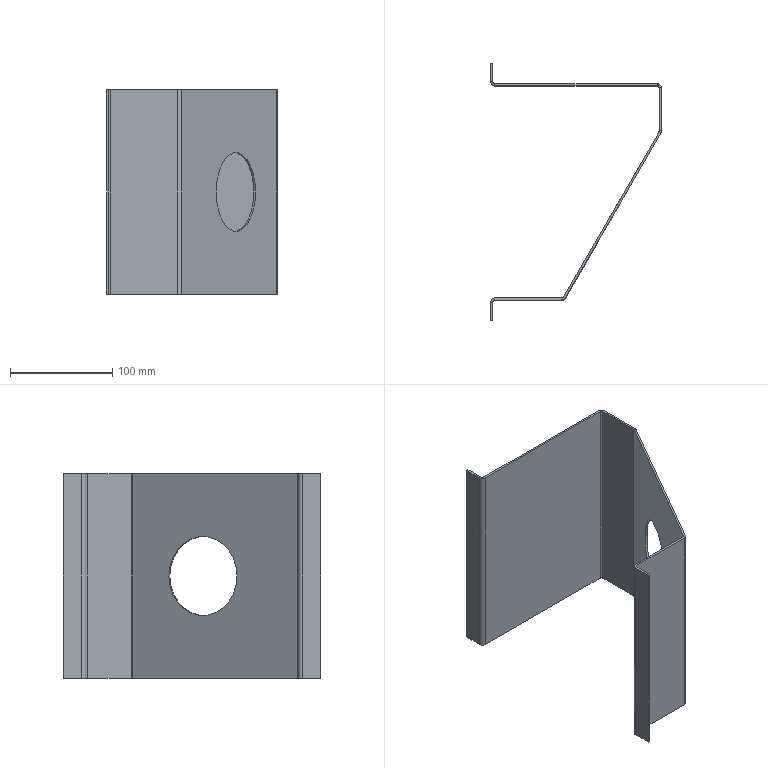Part | STEP file | SYL0380DJ1008_2_7_2_1-2_STEP | 1 solid | 48 faces | box 167 x 252 x 200 mm | volume 194104 mm3 | plane 36 | cylinder 12 | commonest cylinder face diameters 4 x5 8 x5 77 x2
STEP:
#1=CARTESIAN_POINT('',(105.214,80.993,0.));
#2=VERTEX_POINT('',#1);
#3=CARTESIAN_POINT('',(103.482,81.993,0.));
#4=VERTEX_POINT('',#3);
#5=CARTESIAN_POINT('',(103.482,81.993,0.));
#6=DIRECTION('',(-0.866,0.5,0.));
#7=VECTOR('',#6,1000.);
#8=LINE('',#5,#7);
#9=EDGE_CURVE('',#2,#4,#8,.T.);
#10=ORIENTED_EDGE('',*,*,#9,.F.);
#11=CARTESIAN_POINT('',(143.714,147.677,0.));
#12=VERTEX_POINT('',#11);
#13=CARTESIAN_POINT('',(124.464,114.335,0.));
#14=DIRECTION('',(0.866,-0.5,0.));
#15=DIRECTION('',(0.5,0.866,0.));
#16=AXIS2_PLACEMENT_3D('',#13,#14,#15);
#17=CIRCLE('',#16,38.5);
#18=EDGE_CURVE('',#2,#12,#17,.T.);
#19=ORIENTED_EDGE('',*,*,#18,.T.);
#20=CARTESIAN_POINT('',(141.982,148.677,0.));
#21=VERTEX_POINT('',#20);
#22=CARTESIAN_POINT('',(141.982,148.677,0.));
#23=DIRECTION('',(-0.866,0.5,0.));
#24=VECTOR('',#23,1000.);
#25=LINE('',#22,#24);
#26=EDGE_CURVE('',#12,#21,#25,.T.);
#27=ORIENTED_EDGE('',*,*,#26,.T.);
#28=CARTESIAN_POINT('',(122.732,115.335,0.));
#29=DIRECTION('',(0.866,-0.5,0.));
#30=DIRECTION('',(-0.5,-0.866,0.));
#31=AXIS2_PLACEMENT_3D('',#28,#29,#30);
#32=CIRCLE('',#31,38.5);
#33=EDGE_CURVE('',#4,#21,#32,.T.);
#34=ORIENTED_EDGE('',*,*,#33,.F.);
#35=EDGE_LOOP('',(#10,#19,#27,#34));
#36=FACE_OUTER_BOUND('',#35,.T.);
#37=CARTESIAN_POINT('',(122.732,115.335,0.));
#38=DIRECTION('',(0.866,-0.5,0.));
#39=DIRECTION('',(0.5,0.866,0.));
#40=AXIS2_PLACEMENT_3D('',#37,#38,#39);
#41=CYLINDRICAL_SURFACE('',#40,38.5);
#42=ADVANCED_FACE('',(#36),#41,.F.);
#43=CARTESIAN_POINT('',(161.,232.,-100.));
#44=VERTEX_POINT('',#43);
#45=CARTESIAN_POINT('',(161.,230.,-100.));
#46=VERTEX_POINT('',#45);
#47=CARTESIAN_POINT('',(161.,230.,-100.));
#48=DIRECTION('',(0.,-1.,0.));
#49=VECTOR('',#48,1000.);
#50=LINE('',#47,#49);
#51=EDGE_CURVE('',#44,#46,#50,.T.);
#52=ORIENTED_EDGE('',*,*,#51,.F.);
#53=CARTESIAN_POINT('',(165.,228.,-100.));
#54=VERTEX_POINT('',#53);
#55=CARTESIAN_POINT('',(161.,228.,-100.));
#56=DIRECTION('',(0.,0.,1.));
#57=DIRECTION('',(-1.,0.,0.));
#58=AXIS2_PLACEMENT_3D('',#55,#56,#57);
#59=CIRCLE('',#58,4.);
#60=EDGE_CURVE('',#54,#44,#59,.T.);
#61=ORIENTED_EDGE('',*,*,#60,.F.);
#62=CARTESIAN_POINT('',(163.,228.,-100.));
#63=VERTEX_POINT('',#62);
#64=CARTESIAN_POINT('',(163.,228.,-100.));
#65=DIRECTION('',(-1.,0.,0.));
#66=VECTOR('',#65,1000.);
#67=LINE('',#64,#66);
#68=EDGE_CURVE('',#54,#63,#67,.T.);
#69=ORIENTED_EDGE('',*,*,#68,.T.);
#70=CARTESIAN_POINT('',(161.,228.,-100.));
#71=DIRECTION('',(0.,0.,1.));
#72=DIRECTION('',(1.,0.,0.));
#73=AXIS2_PLACEMENT_3D('',#70,#71,#72);
#74=CIRCLE('',#73,2.);
#75=EDGE_CURVE('',#63,#46,#74,.T.);
#76=ORIENTED_EDGE('',*,*,#75,.T.);
#77=EDGE_LOOP('',(#52,#61,#69,#76));
#78=FACE_OUTER_BOUND('',#77,.T.);
#79=CARTESIAN_POINT('',(161.,228.,-100.));
#80=DIRECTION('',(0.,0.,-1.));
#81=DIRECTION('',(-1.,0.,0.));
#82=AXIS2_PLACEMENT_3D('',#79,#80,#81);
#83=PLANE('',#82);
#84=ADVANCED_FACE('',(#78),#83,.T.);
#85=ORIENTED_EDGE('',*,*,#68,.F.);
#86=CARTESIAN_POINT('',(165.,185.617,-100.));
#87=VERTEX_POINT('',#86);
#88=CARTESIAN_POINT('',(165.,184.545,-100.));
#89=DIRECTION('',(0.,-1.,0.));
#90=VECTOR('',#89,1000.);
#91=LINE('',#88,#90);
#92=EDGE_CURVE('',#54,#87,#91,.T.);
#93=ORIENTED_EDGE('',*,*,#92,.T.);
#94=CARTESIAN_POINT('',(163.,185.617,-100.));
#95=VERTEX_POINT('',#94);
#96=CARTESIAN_POINT('',(163.,185.617,-100.));
#97=DIRECTION('',(-1.,0.,0.));
#98=VECTOR('',#97,1000.);
#99=LINE('',#96,#98);
#100=EDGE_CURVE('',#87,#95,#99,.T.);
#101=ORIENTED_EDGE('',*,*,#100,.T.);
#102=CARTESIAN_POINT('',(163.,228.,-100.));
#103=DIRECTION('',(0.,-1.,0.));
#104=VECTOR('',#103,1000.);
#105=LINE('',#102,#104);
#106=EDGE_CURVE('',#63,#95,#105,.T.);
#107=ORIENTED_EDGE('',*,*,#106,.F.);
#108=EDGE_LOOP('',(#85,#93,#101,#107));
#109=FACE_OUTER_BOUND('',#108,.T.);
#110=CARTESIAN_POINT('',(163.,228.,-100.));
#111=DIRECTION('',(0.,0.,1.));
#112=DIRECTION('',(0.,-1.,0.));
#113=AXIS2_PLACEMENT_3D('',#110,#111,#112);
#114=PLANE('',#113);
#115=ADVANCED_FACE('',(#109),#114,.F.);
#116=ORIENTED_EDGE('',*,*,#100,.F.);
#117=CARTESIAN_POINT('',(164.464,183.617,-100.));
#118=VERTEX_POINT('',#117);
#119=CARTESIAN_POINT('',(161.,185.617,-100.));
#120=DIRECTION('',(0.,0.,1.));
#121=DIRECTION('',(-1.,0.,0.));
#122=AXIS2_PLACEMENT_3D('',#119,#120,#121);
#123=CIRCLE('',#122,4.);
#124=EDGE_CURVE('',#118,#87,#123,.T.);
#125=ORIENTED_EDGE('',*,*,#124,.F.);
#126=CARTESIAN_POINT('',(162.732,184.617,-100.));
#127=VERTEX_POINT('',#126);
#128=CARTESIAN_POINT('',(162.732,184.617,-100.));
#129=DIRECTION('',(-0.866,0.5,0.));
#130=VECTOR('',#129,1000.);
#131=LINE('',#128,#130);
#132=EDGE_CURVE('',#118,#127,#131,.T.);
#133=ORIENTED_EDGE('',*,*,#132,.T.);
#134=CARTESIAN_POINT('',(161.,185.617,-100.));
#135=DIRECTION('',(0.,0.,1.));
#136=DIRECTION('',(0.866,-0.5,0.));
#137=AXIS2_PLACEMENT_3D('',#134,#135,#136);
#138=CIRCLE('',#137,2.);
#139=EDGE_CURVE('',#127,#95,#138,.T.);
#140=ORIENTED_EDGE('',*,*,#139,.T.);
#141=EDGE_LOOP('',(#116,#125,#133,#140));
#142=FACE_OUTER_BOUND('',#141,.T.);
#143=CARTESIAN_POINT('',(161.,185.617,-100.));
#144=DIRECTION('',(0.,0.,-1.));
#145=DIRECTION('',(-1.,0.,0.));
#146=AXIS2_PLACEMENT_3D('',#143,#144,#145);
#147=PLANE('',#146);
#148=ADVANCED_FACE('',(#142),#147,.T.);
#149=ORIENTED_EDGE('',*,*,#132,.F.);
#150=CARTESIAN_POINT('',(71.155,22.,-100.));
#151=VERTEX_POINT('',#150);
#152=CARTESIAN_POINT('',(70.,20.,-100.));
#153=DIRECTION('',(0.5,0.866,0.));
#154=VECTOR('',#153,1000.);
#155=LINE('',#152,#154);
#156=EDGE_CURVE('',#151,#118,#155,.T.);
#157=ORIENTED_EDGE('',*,*,#156,.F.);
#158=CARTESIAN_POINT('',(69.423,23.,-100.));
#159=VERTEX_POINT('',#158);
#160=CARTESIAN_POINT('',(69.423,23.,-100.));
#161=DIRECTION('',(-0.866,0.5,0.));
#162=VECTOR('',#161,1000.);
#163=LINE('',#160,#162);
#164=EDGE_CURVE('',#151,#159,#163,.T.);
#165=ORIENTED_EDGE('',*,*,#164,.T.);
#166=CARTESIAN_POINT('',(69.423,23.,-100.));
#167=DIRECTION('',(0.5,0.866,0.));
#168=VECTOR('',#167,1000.);
#169=LINE('',#166,#168);
#170=EDGE_CURVE('',#159,#127,#169,.T.);
#171=ORIENTED_EDGE('',*,*,#170,.T.);
#172=EDGE_LOOP('',(#149,#157,#165,#171));
#173=FACE_OUTER_BOUND('',#172,.T.);
#174=CARTESIAN_POINT('',(69.423,23.,-100.));
#175=DIRECTION('',(0.,0.,-1.));
#176=DIRECTION('',(0.5,0.866,0.));
#177=AXIS2_PLACEMENT_3D('',#174,#175,#176);
#178=PLANE('',#177);
#179=ADVANCED_FACE('',(#173),#178,.T.);
#180=ORIENTED_EDGE('',*,*,#164,.F.);
#181=CARTESIAN_POINT('',(67.691,20.,-100.));
#182=VERTEX_POINT('',#181);
#183=CARTESIAN_POINT('',(67.691,24.,-100.));
#184=DIRECTION('',(0.,0.,1.));
#185=DIRECTION('',(-1.,0.,0.));
#186=AXIS2_PLACEMENT_3D('',#183,#184,#185);
#187=CIRCLE('',#186,4.);
#188=EDGE_CURVE('',#182,#151,#187,.T.);
#189=ORIENTED_EDGE('',*,*,#188,.F.);
#190=CARTESIAN_POINT('',(67.691,22.,-100.));
#191=VERTEX_POINT('',#190);
#192=CARTESIAN_POINT('',(67.691,22.,-100.));
#193=DIRECTION('',(0.,1.,0.));
#194=VECTOR('',#193,1000.);
#195=LINE('',#192,#194);
#196=EDGE_CURVE('',#182,#191,#195,.T.);
#197=ORIENTED_EDGE('',*,*,#196,.T.);
#198=CARTESIAN_POINT('',(67.691,24.,-100.));
#199=DIRECTION('',(0.,0.,1.));
#200=DIRECTION('',(0.,-1.,0.));
#201=AXIS2_PLACEMENT_3D('',#198,#199,#200);
#202=CIRCLE('',#201,2.);
#203=EDGE_CURVE('',#191,#159,#202,.T.);
#204=ORIENTED_EDGE('',*,*,#203,.T.);
#205=EDGE_LOOP('',(#180,#189,#197,#204));
#206=FACE_OUTER_BOUND('',#205,.T.);
#207=CARTESIAN_POINT('',(67.691,24.,-100.));
#208=DIRECTION('',(0.,0.,-1.));
#209=DIRECTION('',(-1.,0.,0.));
#210=AXIS2_PLACEMENT_3D('',#207,#208,#209);
#211=PLANE('',#210);
#212=ADVANCED_FACE('',(#206),#211,.T.);
#213=ORIENTED_EDGE('',*,*,#196,.F.);
#214=CARTESIAN_POINT('',(2.,20.,-100.));
#215=VERTEX_POINT('',#214);
#216=CARTESIAN_POINT('',(0.,20.,-100.));
#217=DIRECTION('',(-1.,0.,0.));
#218=VECTOR('',#217,1000.);
#219=LINE('',#216,#218);
#220=EDGE_CURVE('',#182,#215,#219,.T.);
#221=ORIENTED_EDGE('',*,*,#220,.T.);
#222=CARTESIAN_POINT('',(2.,22.,-100.));
#223=VERTEX_POINT('',#222);
#224=CARTESIAN_POINT('',(2.,22.,-100.));
#225=DIRECTION('',(0.,1.,0.));
#226=VECTOR('',#225,1000.);
#227=LINE('',#224,#226);
#228=EDGE_CURVE('',#215,#223,#227,.T.);
#229=ORIENTED_EDGE('',*,*,#228,.T.);
#230=CARTESIAN_POINT('',(67.691,22.,-100.));
#231=DIRECTION('',(-1.,0.,0.));
#232=VECTOR('',#231,1000.);
#233=LINE('',#230,#232);
#234=EDGE_CURVE('',#191,#223,#233,.T.);
#235=ORIENTED_EDGE('',*,*,#234,.F.);
#236=EDGE_LOOP('',(#213,#221,#229,#235));
#237=FACE_OUTER_BOUND('',#236,.T.);
#238=CARTESIAN_POINT('',(67.691,22.,-100.));
#239=DIRECTION('',(0.,0.,1.));
#240=DIRECTION('',(-1.,0.,0.));
#241=AXIS2_PLACEMENT_3D('',#238,#239,#240);
#242=PLANE('',#241);
#243=ADVANCED_FACE('',(#237),#242,.F.);
#244=ORIENTED_EDGE('',*,*,#228,.F.);
#245=CARTESIAN_POINT('',(0.,18.,-100.));
#246=VERTEX_POINT('',#245);
#247=CARTESIAN_POINT('',(2.,18.,-100.));
#248=DIRECTION('',(0.,0.,-1.));
#249=DIRECTION('',(1.,0.,0.));
#250=AXIS2_PLACEMENT_3D('',#247,#248,#249);
#251=CIRCLE('',#250,2.);
#252=EDGE_CURVE('',#246,#215,#251,.T.);
#253=ORIENTED_EDGE('',*,*,#252,.F.);
#254=CARTESIAN_POINT('',(-2.,18.,-100.));
#255=VERTEX_POINT('',#254);
#256=CARTESIAN_POINT('',(-2.,18.,-100.));
#257=DIRECTION('',(-1.,0.,0.));
#258=VECTOR('',#257,1000.);
#259=LINE('',#256,#258);
#260=EDGE_CURVE('',#246,#255,#259,.T.);
#261=ORIENTED_EDGE('',*,*,#260,.T.);
#262=CARTESIAN_POINT('',(2.,18.,-100.));
#263=DIRECTION('',(0.,0.,-1.));
#264=DIRECTION('',(-1.,0.,0.));
#265=AXIS2_PLACEMENT_3D('',#262,#263,#264);
#266=CIRCLE('',#265,4.);
#267=EDGE_CURVE('',#255,#223,#266,.T.);
#268=ORIENTED_EDGE('',*,*,#267,.T.);
#269=EDGE_LOOP('',(#244,#253,#261,#268));
#270=FACE_OUTER_BOUND('',#269,.T.);
#271=CARTESIAN_POINT('',(2.,18.,-100.));
#272=DIRECTION('',(0.,0.,1.));
#273=DIRECTION('',(1.,0.,0.));
#274=AXIS2_PLACEMENT_3D('',#271,#272,#273);
#275=PLANE('',#274);
#276=ADVANCED_FACE('',(#270),#275,.F.);
#277=ORIENTED_EDGE('',*,*,#260,.F.);
#278=CARTESIAN_POINT('',(0.,0.,-100.));
#279=VERTEX_POINT('',#278);
#280=CARTESIAN_POINT('',(0.,0.,-100.));
#281=DIRECTION('',(0.,-1.,0.));
#282=VECTOR('',#281,1000.);
#283=LINE('',#280,#282);
#284=EDGE_CURVE('',#246,#279,#283,.T.);
#285=ORIENTED_EDGE('',*,*,#284,.T.);
#286=CARTESIAN_POINT('',(-2.,0.,-100.));
#287=VERTEX_POINT('',#286);
#288=CARTESIAN_POINT('',(-2.,0.,-100.));
#289=DIRECTION('',(-1.,0.,0.));
#290=VECTOR('',#289,1000.);
#291=LINE('',#288,#290);
#292=EDGE_CURVE('',#279,#287,#291,.T.);
#293=ORIENTED_EDGE('',*,*,#292,.T.);
#294=CARTESIAN_POINT('',(-2.,18.,-100.));
#295=DIRECTION('',(0.,-1.,0.));
#296=VECTOR('',#295,1000.);
#297=LINE('',#294,#296);
#298=EDGE_CURVE('',#255,#287,#297,.T.);
#299=ORIENTED_EDGE('',*,*,#298,.F.);
#300=EDGE_LOOP('',(#277,#285,#293,#299));
#301=FACE_OUTER_BOUND('',#300,.T.);
#302=CARTESIAN_POINT('',(-2.,18.,-100.));
#303=DIRECTION('',(0.,0.,1.));
#304=DIRECTION('',(0.,-1.,0.));
#305=AXIS2_PLACEMENT_3D('',#302,#303,#304);
#306=PLANE('',#305);
#307=ADVANCED_FACE('',(#301),#306,.F.);
#308=ORIENTED_EDGE('',*,*,#292,.F.);
#309=CARTESIAN_POINT('',(0.,0.,100.));
#310=VERTEX_POINT('',#309);
#311=CARTESIAN_POINT('',(0.,0.,100.));
#312=DIRECTION('',(0.,0.,1.));
#313=VECTOR('',#312,1000.);
#314=LINE('',#311,#313);
#315=EDGE_CURVE('',#279,#310,#314,.T.);
#316=ORIENTED_EDGE('',*,*,#315,.T.);
#317=CARTESIAN_POINT('',(-2.,0.,100.));
#318=VERTEX_POINT('',#317);
#319=CARTESIAN_POINT('',(-2.,0.,100.));
#320=DIRECTION('',(-1.,0.,0.));
#321=VECTOR('',#320,1000.);
#322=LINE('',#319,#321);
#323=EDGE_CURVE('',#310,#318,#322,.T.);
#324=ORIENTED_EDGE('',*,*,#323,.T.);
#325=CARTESIAN_POINT('',(-2.,0.,-100.));
#326=DIRECTION('',(0.,0.,1.));
#327=VECTOR('',#326,1000.);
#328=LINE('',#325,#327);
#329=EDGE_CURVE('',#287,#318,#328,.T.);
#330=ORIENTED_EDGE('',*,*,#329,.F.);
#331=EDGE_LOOP('',(#308,#316,#324,#330));
#332=FACE_OUTER_BOUND('',#331,.T.);
#333=CARTESIAN_POINT('',(-2.,0.,-100.));
#334=DIRECTION('',(0.,1.,0.));
#335=DIRECTION('',(0.,0.,1.));
#336=AXIS2_PLACEMENT_3D('',#333,#334,#335);
#337=PLANE('',#336);
#338=ADVANCED_FACE('',(#332),#337,.F.);
#339=ORIENTED_EDGE('',*,*,#323,.F.);
#340=CARTESIAN_POINT('',(0.,18.,100.));
#341=VERTEX_POINT('',#340);
#342=CARTESIAN_POINT('',(0.,0.,100.));
#343=DIRECTION('',(0.,1.,0.));
#344=VECTOR('',#343,1000.);
#345=LINE('',#342,#344);
#346=EDGE_CURVE('',#310,#341,#345,.T.);
#347=ORIENTED_EDGE('',*,*,#346,.T.);
#348=CARTESIAN_POINT('',(-2.,18.,100.));
#349=VERTEX_POINT('',#348);
#350=CARTESIAN_POINT('',(-2.,18.,100.));
#351=DIRECTION('',(-1.,0.,0.));
#352=VECTOR('',#351,1000.);
#353=LINE('',#350,#352);
#354=EDGE_CURVE('',#341,#349,#353,.T.);
#355=ORIENTED_EDGE('',*,*,#354,.T.);
#356=CARTESIAN_POINT('',(-2.,0.,100.));
#357=DIRECTION('',(0.,1.,0.));
#358=VECTOR('',#357,1000.);
#359=LINE('',#356,#358);
#360=EDGE_CURVE('',#318,#349,#359,.T.);
#361=ORIENTED_EDGE('',*,*,#360,.F.);
#362=EDGE_LOOP('',(#339,#347,#355,#361));
#363=FACE_OUTER_BOUND('',#362,.T.);
#364=CARTESIAN_POINT('',(-2.,0.,100.));
#365=DIRECTION('',(0.,0.,-1.));
#366=DIRECTION('',(0.,1.,0.));
#367=AXIS2_PLACEMENT_3D('',#364,#365,#366);
#368=PLANE('',#367);
#369=ADVANCED_FACE('',(#363),#368,.F.);
#370=ORIENTED_EDGE('',*,*,#354,.F.);
#371=CARTESIAN_POINT('',(2.,20.,100.));
#372=VERTEX_POINT('',#371);
#373=CARTESIAN_POINT('',(2.,18.,100.));
#374=DIRECTION('',(0.,0.,1.));
#375=DIRECTION('',(1.,0.,0.));
#376=AXIS2_PLACEMENT_3D('',#373,#374,#375);
#377=CIRCLE('',#376,2.);
#378=EDGE_CURVE('',#372,#341,#377,.T.);
#379=ORIENTED_EDGE('',*,*,#378,.F.);
#380=CARTESIAN_POINT('',(2.,22.,100.));
#381=VERTEX_POINT('',#380);
#382=CARTESIAN_POINT('',(2.,22.,100.));
#383=DIRECTION('',(0.,1.,0.));
#384=VECTOR('',#383,1000.);
#385=LINE('',#382,#384);
#386=EDGE_CURVE('',#372,#381,#385,.T.);
#387=ORIENTED_EDGE('',*,*,#386,.T.);
#388=CARTESIAN_POINT('',(2.,18.,100.));
#389=DIRECTION('',(0.,0.,1.));
#390=DIRECTION('',(0.,1.,0.));
#391=AXIS2_PLACEMENT_3D('',#388,#389,#390);
#392=CIRCLE('',#391,4.);
#393=EDGE_CURVE('',#381,#349,#392,.T.);
#394=ORIENTED_EDGE('',*,*,#393,.T.);
#395=EDGE_LOOP('',(#370,#379,#387,#394));
#396=FACE_OUTER_BOUND('',#395,.T.);
#397=CARTESIAN_POINT('',(2.,18.,100.));
#398=DIRECTION('',(0.,0.,-1.));
#399=DIRECTION('',(-1.,0.,0.));
#400=AXIS2_PLACEMENT_3D('',#397,#398,#399);
#401=PLANE('',#400);
#402=ADVANCED_FACE('',(#396),#401,.F.);
#403=ORIENTED_EDGE('',*,*,#386,.F.);
#404=CARTESIAN_POINT('',(67.691,20.,100.));
#405=VERTEX_POINT('',#404);
#406=CARTESIAN_POINT('',(0.,20.,100.));
#407=DIRECTION('',(1.,0.,0.));
#408=VECTOR('',#407,1000.);
#409=LINE('',#406,#408);
#410=EDGE_CURVE('',#372,#405,#409,.T.);
#411=ORIENTED_EDGE('',*,*,#410,.T.);
#412=CARTESIAN_POINT('',(67.691,22.,100.));
#413=VERTEX_POINT('',#412);
#414=CARTESIAN_POINT('',(67.691,22.,100.));
#415=DIRECTION('',(0.,1.,0.));
#416=VECTOR('',#415,1000.);
#417=LINE('',#414,#416);
#418=EDGE_CURVE('',#405,#413,#417,.T.);
#419=ORIENTED_EDGE('',*,*,#418,.T.);
#420=CARTESIAN_POINT('',(2.,22.,100.));
#421=DIRECTION('',(1.,0.,0.));
#422=VECTOR('',#421,1000.);
#423=LINE('',#420,#422);
#424=EDGE_CURVE('',#381,#413,#423,.T.);
#425=ORIENTED_EDGE('',*,*,#424,.F.);
#426=EDGE_LOOP('',(#403,#411,#419,#425));
#427=FACE_OUTER_BOUND('',#426,.T.);
#428=CARTESIAN_POINT('',(2.,22.,100.));
#429=DIRECTION('',(0.,0.,-1.));
#430=DIRECTION('',(1.,0.,0.));
#431=AXIS2_PLACEMENT_3D('',#428,#429,#430);
#432=PLANE('',#431);
#433=ADVANCED_FACE('',(#427),#432,.F.);
#434=ORIENTED_EDGE('',*,*,#418,.F.);
#435=CARTESIAN_POINT('',(71.155,22.,100.));
#436=VERTEX_POINT('',#435);
#437=CARTESIAN_POINT('',(67.691,24.,100.));
#438=DIRECTION('',(0.,0.,-1.));
#439=DIRECTION('',(-1.,0.,0.));
#440=AXIS2_PLACEMENT_3D('',#437,#438,#439);
#441=CIRCLE('',#440,4.);
#442=EDGE_CURVE('',#436,#405,#441,.T.);
#443=ORIENTED_EDGE('',*,*,#442,.F.);
#444=CARTESIAN_POINT('',(69.423,23.,100.));
#445=VERTEX_POINT('',#444);
#446=CARTESIAN_POINT('',(69.423,23.,100.));
#447=DIRECTION('',(-0.866,0.5,0.));
#448=VECTOR('',#447,1000.);
#449=LINE('',#446,#448);
#450=EDGE_CURVE('',#436,#445,#449,.T.);
#451=ORIENTED_EDGE('',*,*,#450,.T.);
#452=CARTESIAN_POINT('',(67.691,24.,100.));
#453=DIRECTION('',(0.,0.,-1.));
#454=DIRECTION('',(0.866,-0.5,0.));
#455=AXIS2_PLACEMENT_3D('',#452,#453,#454);
#456=CIRCLE('',#455,2.);
#457=EDGE_CURVE('',#445,#413,#456,.T.);
#458=ORIENTED_EDGE('',*,*,#457,.T.);
#459=EDGE_LOOP('',(#434,#443,#451,#458));
#460=FACE_OUTER_BOUND('',#459,.T.);
#461=CARTESIAN_POINT('',(67.691,24.,100.));
#462=DIRECTION('',(0.,0.,1.));
#463=DIRECTION('',(1.,0.,0.));
#464=AXIS2_PLACEMENT_3D('',#461,#462,#463);
#465=PLANE('',#464);
#466=ADVANCED_FACE('',(#460),#465,.T.);
#467=ORIENTED_EDGE('',*,*,#450,.F.);
#468=CARTESIAN_POINT('',(164.464,183.617,100.));
#469=VERTEX_POINT('',#468);
#470=CARTESIAN_POINT('',(70.,20.,100.));
#471=DIRECTION('',(-0.5,-0.866,0.));
#472=VECTOR('',#471,1000.);
#473=LINE('',#470,#472);
#474=EDGE_CURVE('',#469,#436,#473,.T.);
#475=ORIENTED_EDGE('',*,*,#474,.F.);
#476=CARTESIAN_POINT('',(162.732,184.617,100.));
#477=VERTEX_POINT('',#476);
#478=CARTESIAN_POINT('',(162.732,184.617,100.));
#479=DIRECTION('',(-0.866,0.5,0.));
#480=VECTOR('',#479,1000.);
#481=LINE('',#478,#480);
#482=EDGE_CURVE('',#469,#477,#481,.T.);
#483=ORIENTED_EDGE('',*,*,#482,.T.);
#484=CARTESIAN_POINT('',(162.732,184.617,100.));
#485=DIRECTION('',(-0.5,-0.866,0.));
#486=VECTOR('',#485,1000.);
#487=LINE('',#484,#486);
#488=EDGE_CURVE('',#477,#445,#487,.T.);
#489=ORIENTED_EDGE('',*,*,#488,.T.);
#490=EDGE_LOOP('',(#467,#475,#483,#489));
#491=FACE_OUTER_BOUND('',#490,.T.);
#492=CARTESIAN_POINT('',(162.732,184.617,100.));
#493=DIRECTION('',(0.,0.,1.));
#494=DIRECTION('',(-0.5,-0.866,0.));
#495=AXIS2_PLACEMENT_3D('',#492,#493,#494);
#496=PLANE('',#495);
#497=ADVANCED_FACE('',(#491),#496,.T.);
#498=ORIENTED_EDGE('',*,*,#482,.F.);
#499=CARTESIAN_POINT('',(165.,185.617,100.));
#500=VERTEX_POINT('',#499);
#501=CARTESIAN_POINT('',(161.,185.617,100.));
#502=DIRECTION('',(0.,0.,-1.));
#503=DIRECTION('',(-1.,0.,0.));
#504=AXIS2_PLACEMENT_3D('',#501,#502,#503);
#505=CIRCLE('',#504,4.);
#506=EDGE_CURVE('',#500,#469,#505,.T.);
#507=ORIENTED_EDGE('',*,*,#506,.F.);
#508=CARTESIAN_POINT('',(163.,185.617,100.));
#509=VERTEX_POINT('',#508);
#510=CARTESIAN_POINT('',(163.,185.617,100.));
#511=DIRECTION('',(-1.,0.,0.));
#512=VECTOR('',#511,1000.);
#513=LINE('',#510,#512);
#514=EDGE_CURVE('',#500,#509,#513,.T.);
#515=ORIENTED_EDGE('',*,*,#514,.T.);
#516=CARTESIAN_POINT('',(161.,185.617,100.));
#517=DIRECTION('',(0.,0.,-1.));
#518=DIRECTION('',(1.,0.,0.));
#519=AXIS2_PLACEMENT_3D('',#516,#517,#518);
#520=CIRCLE('',#519,2.);
#521=EDGE_CURVE('',#509,#477,#520,.T.);
#522=ORIENTED_EDGE('',*,*,#521,.T.);
#523=EDGE_LOOP('',(#498,#507,#515,#522));
#524=FACE_OUTER_BOUND('',#523,.T.);
#525=CARTESIAN_POINT('',(161.,185.617,100.));
#526=DIRECTION('',(0.,0.,1.));
#527=DIRECTION('',(1.,0.,0.));
#528=AXIS2_PLACEMENT_3D('',#525,#526,#527);
#529=PLANE('',#528);
#530=ADVANCED_FACE('',(#524),#529,.T.);
#531=ORIENTED_EDGE('',*,*,#514,.F.);
#532=CARTESIAN_POINT('',(165.,228.,100.));
#533=VERTEX_POINT('',#532);
#534=CARTESIAN_POINT('',(165.,184.545,100.));
#535=DIRECTION('',(0.,1.,0.));
#536=VECTOR('',#535,1000.);
#537=LINE('',#534,#536);
#538=EDGE_CURVE('',#500,#533,#537,.T.);
#539=ORIENTED_EDGE('',*,*,#538,.T.);
#540=CARTESIAN_POINT('',(163.,228.,100.));
#541=VERTEX_POINT('',#540);
#542=CARTESIAN_POINT('',(163.,228.,100.));
#543=DIRECTION('',(-1.,0.,0.));
#544=VECTOR('',#543,1000.);
#545=LINE('',#542,#544);
#546=EDGE_CURVE('',#533,#541,#545,.T.);
#547=ORIENTED_EDGE('',*,*,#546,.T.);
#548=CARTESIAN_POINT('',(163.,185.617,100.));
#549=DIRECTION('',(0.,1.,0.));
#550=VECTOR('',#549,1000.);
#551=LINE('',#548,#550);
#552=EDGE_CURVE('',#509,#541,#551,.T.);
#553=ORIENTED_EDGE('',*,*,#552,.F.);
#554=EDGE_LOOP('',(#531,#539,#547,#553));
#555=FACE_OUTER_BOUND('',#554,.T.);
#556=CARTESIAN_POINT('',(163.,185.617,100.));
#557=DIRECTION('',(0.,0.,-1.));
#558=DIRECTION('',(0.,1.,0.));
#559=AXIS2_PLACEMENT_3D('',#556,#557,#558);
#560=PLANE('',#559);
#561=ADVANCED_FACE('',(#555),#560,.F.);
#562=ORIENTED_EDGE('',*,*,#546,.F.);
#563=CARTESIAN_POINT('',(161.,232.,100.));
#564=VERTEX_POINT('',#563);
#565=CARTESIAN_POINT('',(161.,228.,100.));
#566=DIRECTION('',(0.,0.,-1.));
#567=DIRECTION('',(-1.,0.,0.));
#568=AXIS2_PLACEMENT_3D('',#565,#566,#567);
#569=CIRCLE('',#568,4.);
#570=EDGE_CURVE('',#564,#533,#569,.T.);
#571=ORIENTED_EDGE('',*,*,#570,.F.);
#572=CARTESIAN_POINT('',(161.,230.,100.));
#573=VERTEX_POINT('',#572);
#574=CARTESIAN_POINT('',(161.,230.,100.));
#575=DIRECTION('',(0.,-1.,0.));
#576=VECTOR('',#575,1000.);
#577=LINE('',#574,#576);
#578=EDGE_CURVE('',#564,#573,#577,.T.);
#579=ORIENTED_EDGE('',*,*,#578,.T.);
#580=CARTESIAN_POINT('',(161.,228.,100.));
#581=DIRECTION('',(0.,0.,-1.));
#582=DIRECTION('',(0.,1.,0.));
#583=AXIS2_PLACEMENT_3D('',#580,#581,#582);
#584=CIRCLE('',#583,2.);
#585=EDGE_CURVE('',#573,#541,#584,.T.);
#586=ORIENTED_EDGE('',*,*,#585,.T.);
#587=EDGE_LOOP('',(#562,#571,#579,#586));
#588=FACE_OUTER_BOUND('',#587,.T.);
#589=CARTESIAN_POINT('',(161.,228.,100.));
#590=DIRECTION('',(0.,0.,1.));
#591=DIRECTION('',(1.,0.,0.));
#592=AXIS2_PLACEMENT_3D('',#589,#590,#591);
#593=PLANE('',#592);
#594=ADVANCED_FACE('',(#588),#593,.T.);
#595=ORIENTED_EDGE('',*,*,#578,.F.);
#596=CARTESIAN_POINT('',(2.,232.,100.));
#597=VERTEX_POINT('',#596);
#598=CARTESIAN_POINT('',(165.,232.,100.));
#599=DIRECTION('',(-1.,0.,0.));
#600=VECTOR('',#599,1000.);
#601=LINE('',#598,#600);
#602=EDGE_CURVE('',#564,#597,#601,.T.);
#603=ORIENTED_EDGE('',*,*,#602,.T.);
#604=CARTESIAN_POINT('',(2.,230.,100.));
#605=VERTEX_POINT('',#604);
#606=CARTESIAN_POINT('',(2.,230.,100.));
#607=DIRECTION('',(0.,-1.,0.));
#608=VECTOR('',#607,1000.);
#609=LINE('',#606,#608);
#610=EDGE_CURVE('',#597,#605,#609,.T.);
#611=ORIENTED_EDGE('',*,*,#610,.T.);
#612=CARTESIAN_POINT('',(161.,230.,100.));
#613=DIRECTION('',(-1.,0.,0.));
#614=VECTOR('',#613,1000.);
#615=LINE('',#612,#614);
#616=EDGE_CURVE('',#573,#605,#615,.T.);
#617=ORIENTED_EDGE('',*,*,#616,.F.);
#618=EDGE_LOOP('',(#595,#603,#611,#617));
#619=FACE_OUTER_BOUND('',#618,.T.);
#620=CARTESIAN_POINT('',(161.,230.,100.));
#621=DIRECTION('',(0.,0.,-1.));
#622=DIRECTION('',(-1.,0.,0.));
#623=AXIS2_PLACEMENT_3D('',#620,#621,#622);
#624=PLANE('',#623);
#625=ADVANCED_FACE('',(#619),#624,.F.);
#626=ORIENTED_EDGE('',*,*,#610,.F.);
#627=CARTESIAN_POINT('',(0.,234.,100.));
#628=VERTEX_POINT('',#627);
#629=CARTESIAN_POINT('',(2.,234.,100.));
#630=DIRECTION('',(0.,0.,1.));
#631=DIRECTION('',(1.,0.,0.));
#632=AXIS2_PLACEMENT_3D('',#629,#630,#631);
#633=CIRCLE('',#632,2.);
#634=EDGE_CURVE('',#628,#597,#633,.T.);
#635=ORIENTED_EDGE('',*,*,#634,.F.);
#636=CARTESIAN_POINT('',(-2.,234.,100.));
#637=VERTEX_POINT('',#636);
#638=CARTESIAN_POINT('',(-2.,234.,100.));
#639=DIRECTION('',(-1.,0.,0.));
#640=VECTOR('',#639,1000.);
#641=LINE('',#638,#640);
#642=EDGE_CURVE('',#628,#637,#641,.T.);
#643=ORIENTED_EDGE('',*,*,#642,.T.);
#644=CARTESIAN_POINT('',(2.,234.,100.));
#645=DIRECTION('',(0.,0.,1.));
#646=DIRECTION('',(-1.,0.,0.));
#647=AXIS2_PLACEMENT_3D('',#644,#645,#646);
#648=CIRCLE('',#647,4.);
#649=EDGE_CURVE('',#637,#605,#648,.T.);
#650=ORIENTED_EDGE('',*,*,#649,.T.);
#651=EDGE_LOOP('',(#626,#635,#643,#650));
#652=FACE_OUTER_BOUND('',#651,.T.);
#653=CARTESIAN_POINT('',(2.,234.,100.));
#654=DIRECTION('',(0.,0.,-1.));
#655=DIRECTION('',(-1.,0.,0.));
#656=AXIS2_PLACEMENT_3D('',#653,#654,#655);
#657=PLANE('',#656);
#658=ADVANCED_FACE('',(#652),#657,.F.);
#659=ORIENTED_EDGE('',*,*,#642,.F.);
#660=CARTESIAN_POINT('',(0.,252.,100.));
#661=VERTEX_POINT('',#660);
#662=CARTESIAN_POINT('',(0.,232.,100.));
#663=DIRECTION('',(0.,1.,0.));
#664=VECTOR('',#663,1000.);
#665=LINE('',#662,#664);
#666=EDGE_CURVE('',#628,#661,#665,.T.);
#667=ORIENTED_EDGE('',*,*,#666,.T.);
#668=CARTESIAN_POINT('',(-2.,252.,100.));
#669=VERTEX_POINT('',#668);
#670=CARTESIAN_POINT('',(-2.,252.,100.));
#671=DIRECTION('',(-1.,0.,0.));
#672=VECTOR('',#671,1000.);
#673=LINE('',#670,#672);
#674=EDGE_CURVE('',#661,#669,#673,.T.);
#675=ORIENTED_EDGE('',*,*,#674,.T.);
#676=CARTESIAN_POINT('',(-2.,234.,100.));
#677=DIRECTION('',(0.,1.,0.));
#678=VECTOR('',#677,1000.);
#679=LINE('',#676,#678);
#680=EDGE_CURVE('',#637,#669,#679,.T.);
#681=ORIENTED_EDGE('',*,*,#680,.F.);
#682=EDGE_LOOP('',(#659,#667,#675,#681));
#683=FACE_OUTER_BOUND('',#682,.T.);
#684=CARTESIAN_POINT('',(-2.,234.,100.));
#685=DIRECTION('',(0.,0.,-1.));
#686=DIRECTION('',(0.,1.,0.));
#687=AXIS2_PLACEMENT_3D('',#684,#685,#686);
#688=PLANE('',#687);
#689=ADVANCED_FACE('',(#683),#688,.F.);
#690=ORIENTED_EDGE('',*,*,#674,.F.);
#691=CARTESIAN_POINT('',(0.,252.,-100.));
#692=VERTEX_POINT('',#691);
#693=CARTESIAN_POINT('',(0.,252.,100.));
#694=DIRECTION('',(0.,0.,-1.));
#695=VECTOR('',#694,1000.);
#696=LINE('',#693,#695);
#697=EDGE_CURVE('',#661,#692,#696,.T.);
#698=ORIENTED_EDGE('',*,*,#697,.T.);
#699=CARTESIAN_POINT('',(-2.,252.,-100.));
#700=VERTEX_POINT('',#699);
#701=CARTESIAN_POINT('',(-2.,252.,-100.));
#702=DIRECTION('',(-1.,0.,0.));
#703=VECTOR('',#702,1000.);
#704=LINE('',#701,#703);
#705=EDGE_CURVE('',#692,#700,#704,.T.);
#706=ORIENTED_EDGE('',*,*,#705,.T.);
#707=CARTESIAN_POINT('',(-2.,252.,100.));
#708=DIRECTION('',(0.,0.,-1.));
#709=VECTOR('',#708,1000.);
#710=LINE('',#707,#709);
#711=EDGE_CURVE('',#669,#700,#710,.T.);
#712=ORIENTED_EDGE('',*,*,#711,.F.);
#713=EDGE_LOOP('',(#690,#698,#706,#712));
#714=FACE_OUTER_BOUND('',#713,.T.);
#715=CARTESIAN_POINT('',(-2.,252.,100.));
#716=DIRECTION('',(0.,-1.,0.));
#717=DIRECTION('',(0.,0.,-1.));
#718=AXIS2_PLACEMENT_3D('',#715,#716,#717);
#719=PLANE('',#718);
#720=ADVANCED_FACE('',(#714),#719,.F.);
#721=ORIENTED_EDGE('',*,*,#705,.F.);
#722=CARTESIAN_POINT('',(0.,234.,-100.));
#723=VERTEX_POINT('',#722);
#724=CARTESIAN_POINT('',(0.,232.,-100.));
#725=DIRECTION('',(0.,-1.,0.));
#726=VECTOR('',#725,1000.);
#727=LINE('',#724,#726);
#728=EDGE_CURVE('',#692,#723,#727,.T.);
#729=ORIENTED_EDGE('',*,*,#728,.T.);
#730=CARTESIAN_POINT('',(-2.,234.,-100.));
#731=VERTEX_POINT('',#730);
#732=CARTESIAN_POINT('',(-2.,234.,-100.));
#733=DIRECTION('',(-1.,0.,0.));
#734=VECTOR('',#733,1000.);
#735=LINE('',#732,#734);
#736=EDGE_CURVE('',#723,#731,#735,.T.);
#737=ORIENTED_EDGE('',*,*,#736,.T.);
#738=CARTESIAN_POINT('',(-2.,252.,-100.));
#739=DIRECTION('',(0.,-1.,0.));
#740=VECTOR('',#739,1000.);
#741=LINE('',#738,#740);
#742=EDGE_CURVE('',#700,#731,#741,.T.);
#743=ORIENTED_EDGE('',*,*,#742,.F.);
#744=EDGE_LOOP('',(#721,#729,#737,#743));
#745=FACE_OUTER_BOUND('',#744,.T.);
#746=CARTESIAN_POINT('',(-2.,252.,-100.));
#747=DIRECTION('',(0.,0.,1.));
#748=DIRECTION('',(0.,-1.,0.));
#749=AXIS2_PLACEMENT_3D('',#746,#747,#748);
#750=PLANE('',#749);
#751=ADVANCED_FACE('',(#745),#750,.F.);
#752=ORIENTED_EDGE('',*,*,#736,.F.);
#753=CARTESIAN_POINT('',(2.,232.,-100.));
#754=VERTEX_POINT('',#753);
#755=CARTESIAN_POINT('',(2.,234.,-100.));
#756=DIRECTION('',(0.,0.,-1.));
#757=DIRECTION('',(1.,0.,0.));
#758=AXIS2_PLACEMENT_3D('',#755,#756,#757);
#759=CIRCLE('',#758,2.);
#760=EDGE_CURVE('',#754,#723,#759,.T.);
#761=ORIENTED_EDGE('',*,*,#760,.F.);
#762=CARTESIAN_POINT('',(2.,230.,-100.));
#763=VERTEX_POINT('',#762);
#764=CARTESIAN_POINT('',(2.,230.,-100.));
#765=DIRECTION('',(0.,-1.,0.));
#766=VECTOR('',#765,1000.);
#767=LINE('',#764,#766);
#768=EDGE_CURVE('',#754,#763,#767,.T.);
#769=ORIENTED_EDGE('',*,*,#768,.T.);
#770=CARTESIAN_POINT('',(2.,234.,-100.));
#771=DIRECTION('',(0.,0.,-1.));
#772=DIRECTION('',(0.,-1.,0.));
#773=AXIS2_PLACEMENT_3D('',#770,#771,#772);
#774=CIRCLE('',#773,4.);
#775=EDGE_CURVE('',#763,#731,#774,.T.);
#776=ORIENTED_EDGE('',*,*,#775,.T.);
#777=EDGE_LOOP('',(#752,#761,#769,#776));
#778=FACE_OUTER_BOUND('',#777,.T.);
#779=CARTESIAN_POINT('',(2.,234.,-100.));
#780=DIRECTION('',(0.,0.,1.));
#781=DIRECTION('',(1.,0.,0.));
#782=AXIS2_PLACEMENT_3D('',#779,#780,#781);
#783=PLANE('',#782);
#784=ADVANCED_FACE('',(#778),#783,.F.);
#785=CARTESIAN_POINT('',(124.464,114.335,0.));
#786=DIRECTION('',(0.866,-0.5,0.));
#787=DIRECTION('',(0.5,0.866,0.));
#788=AXIS2_PLACEMENT_3D('',#785,#786,#787);
#789=CIRCLE('',#788,38.5);
#790=EDGE_CURVE('',#12,#2,#789,.T.);
#791=ORIENTED_EDGE('',*,*,#790,.T.);
#792=ORIENTED_EDGE('',*,*,#9,.T.);
#793=CARTESIAN_POINT('',(122.732,115.335,0.));
#794=DIRECTION('',(0.866,-0.5,0.));
#795=DIRECTION('',(0.5,0.866,0.));
#796=AXIS2_PLACEMENT_3D('',#793,#794,#795);
#797=CIRCLE('',#796,38.5);
#798=EDGE_CURVE('',#21,#4,#797,.T.);
#799=ORIENTED_EDGE('',*,*,#798,.F.);
#800=ORIENTED_EDGE('',*,*,#26,.F.);
#801=EDGE_LOOP('',(#791,#792,#799,#800));
#802=FACE_OUTER_BOUND('',#801,.T.);
#803=CARTESIAN_POINT('',(122.732,115.335,0.));
#804=DIRECTION('',(0.866,-0.5,0.));
#805=DIRECTION('',(0.5,0.866,0.));
#806=AXIS2_PLACEMENT_3D('',#803,#804,#805);
#807=CYLINDRICAL_SURFACE('',#806,38.5);
#808=ADVANCED_FACE('',(#802),#807,.F.);
#809=CARTESIAN_POINT('',(165.,232.,-100.));
#810=DIRECTION('',(1.,0.,0.));
#811=VECTOR('',#810,1000.);
#812=LINE('',#809,#811);
#813=EDGE_CURVE('',#754,#44,#812,.T.);
#814=ORIENTED_EDGE('',*,*,#813,.T.);
#815=ORIENTED_EDGE('',*,*,#51,.T.);
#816=CARTESIAN_POINT('',(2.,230.,-100.));
#817=DIRECTION('',(1.,0.,0.));
#818=VECTOR('',#817,1000.);
#819=LINE('',#816,#818);
#820=EDGE_CURVE('',#763,#46,#819,.T.);
#821=ORIENTED_EDGE('',*,*,#820,.F.);
#822=ORIENTED_EDGE('',*,*,#768,.F.);
#823=EDGE_LOOP('',(#814,#815,#821,#822));
#824=FACE_OUTER_BOUND('',#823,.T.);
#825=CARTESIAN_POINT('',(2.,230.,-100.));
#826=DIRECTION('',(0.,0.,1.));
#827=DIRECTION('',(1.,0.,0.));
#828=AXIS2_PLACEMENT_3D('',#825,#826,#827);
#829=PLANE('',#828);
#830=ADVANCED_FACE('',(#824),#829,.F.);
#831=CARTESIAN_POINT('',(-2.,234.,100.));
#832=DIRECTION('',(0.,0.,-1.));
#833=VECTOR('',#832,1000.);
#834=LINE('',#831,#833);
#835=EDGE_CURVE('',#637,#731,#834,.T.);
#836=ORIENTED_EDGE('',*,*,#835,.T.);
#837=ORIENTED_EDGE('',*,*,#775,.F.);
#838=CARTESIAN_POINT('',(2.,230.,-100.));
#839=DIRECTION('',(0.,0.,1.));
#840=VECTOR('',#839,1000.);
#841=LINE('',#838,#840);
#842=EDGE_CURVE('',#763,#605,#841,.T.);
#843=ORIENTED_EDGE('',*,*,#842,.T.);
#844=ORIENTED_EDGE('',*,*,#649,.F.);
#845=EDGE_LOOP('',(#836,#837,#843,#844));
#846=FACE_OUTER_BOUND('',#845,.T.);
#847=CARTESIAN_POINT('',(2.,234.,-360.72));
#848=DIRECTION('',(0.,0.,1.));
#849=DIRECTION('',(1.,0.,0.));
#850=AXIS2_PLACEMENT_3D('',#847,#848,#849);
#851=CYLINDRICAL_SURFACE('',#850,4.);
#852=ADVANCED_FACE('',(#846),#851,.T.);
#853=ORIENTED_EDGE('',*,*,#835,.F.);
#854=ORIENTED_EDGE('',*,*,#680,.T.);
#855=ORIENTED_EDGE('',*,*,#711,.T.);
#856=ORIENTED_EDGE('',*,*,#742,.T.);
#857=EDGE_LOOP('',(#853,#854,#855,#856));
#858=FACE_OUTER_BOUND('',#857,.T.);
#859=CARTESIAN_POINT('',(-2.,232.,100.));
#860=DIRECTION('',(1.,0.,0.));
#861=DIRECTION('',(0.,1.,0.));
#862=AXIS2_PLACEMENT_3D('',#859,#860,#861);
#863=PLANE('',#862);
#864=ADVANCED_FACE('',(#858),#863,.F.);
#865=ORIENTED_EDGE('',*,*,#75,.F.);
#866=CARTESIAN_POINT('',(163.,228.,-100.));
#867=DIRECTION('',(0.,0.,1.));
#868=VECTOR('',#867,1000.);
#869=LINE('',#866,#868);
#870=EDGE_CURVE('',#63,#541,#869,.T.);
#871=ORIENTED_EDGE('',*,*,#870,.T.);
#872=ORIENTED_EDGE('',*,*,#585,.F.);
#873=CARTESIAN_POINT('',(161.,230.,100.));
#874=DIRECTION('',(0.,0.,-1.));
#875=VECTOR('',#874,1000.);
#876=LINE('',#873,#875);
#877=EDGE_CURVE('',#573,#46,#876,.T.);
#878=ORIENTED_EDGE('',*,*,#877,.T.);
#879=EDGE_LOOP('',(#865,#871,#872,#878));
#880=FACE_OUTER_BOUND('',#879,.T.);
#881=CARTESIAN_POINT('',(161.,228.,360.72));
#882=DIRECTION('',(0.,0.,-1.));
#883=DIRECTION('',(-1.,0.,0.));
#884=AXIS2_PLACEMENT_3D('',#881,#882,#883);
#885=CYLINDRICAL_SURFACE('',#884,2.);
#886=ADVANCED_FACE('',(#880),#885,.F.);
#887=ORIENTED_EDGE('',*,*,#820,.T.);
#888=ORIENTED_EDGE('',*,*,#877,.F.);
#889=ORIENTED_EDGE('',*,*,#616,.T.);
#890=ORIENTED_EDGE('',*,*,#842,.F.);
#891=EDGE_LOOP('',(#887,#888,#889,#890));
#892=FACE_OUTER_BOUND('',#891,.T.);
#893=CARTESIAN_POINT('',(165.,230.,100.));
#894=DIRECTION('',(0.,1.,0.));
#895=DIRECTION('',(1.,0.,0.));
#896=AXIS2_PLACEMENT_3D('',#893,#894,#895);
#897=PLANE('',#896);
#898=ADVANCED_FACE('',(#892),#897,.F.);
#899=ORIENTED_EDGE('',*,*,#139,.F.);
#900=CARTESIAN_POINT('',(162.732,184.617,-100.));
#901=DIRECTION('',(0.,0.,1.));
#902=VECTOR('',#901,1000.);
#903=LINE('',#900,#902);
#904=EDGE_CURVE('',#127,#477,#903,.T.);
#905=ORIENTED_EDGE('',*,*,#904,.T.);
#906=ORIENTED_EDGE('',*,*,#521,.F.);
#907=CARTESIAN_POINT('',(163.,185.617,100.));
#908=DIRECTION('',(0.,0.,-1.));
#909=VECTOR('',#908,1000.);
#910=LINE('',#907,#909);
#911=EDGE_CURVE('',#509,#95,#910,.T.);
#912=ORIENTED_EDGE('',*,*,#911,.T.);
#913=EDGE_LOOP('',(#899,#905,#906,#912));
#914=FACE_OUTER_BOUND('',#913,.T.);
#915=CARTESIAN_POINT('',(161.,185.617,360.72));
#916=DIRECTION('',(0.,0.,-1.));
#917=DIRECTION('',(-1.,0.,0.));
#918=AXIS2_PLACEMENT_3D('',#915,#916,#917);
#919=CYLINDRICAL_SURFACE('',#918,2.);
#920=ADVANCED_FACE('',(#914),#919,.F.);
#921=ORIENTED_EDGE('',*,*,#552,.T.);
#922=ORIENTED_EDGE('',*,*,#870,.F.);
#923=ORIENTED_EDGE('',*,*,#106,.T.);
#924=ORIENTED_EDGE('',*,*,#911,.F.);
#925=EDGE_LOOP('',(#921,#922,#923,#924));
#926=FACE_OUTER_BOUND('',#925,.T.);
#927=CARTESIAN_POINT('',(163.,184.545,100.));
#928=DIRECTION('',(1.,0.,0.));
#929=DIRECTION('',(0.,1.,0.));
#930=AXIS2_PLACEMENT_3D('',#927,#928,#929);
#931=PLANE('',#930);
#932=ADVANCED_FACE('',(#926),#931,.F.);
#933=CARTESIAN_POINT('',(2.,22.,100.));
#934=DIRECTION('',(0.,0.,-1.));
#935=VECTOR('',#934,1000.);
#936=LINE('',#933,#935);
#937=EDGE_CURVE('',#381,#223,#936,.T.);
#938=ORIENTED_EDGE('',*,*,#937,.T.);
#939=ORIENTED_EDGE('',*,*,#267,.F.);
#940=CARTESIAN_POINT('',(-2.,18.,-100.));
#941=DIRECTION('',(0.,0.,1.));
#942=VECTOR('',#941,1000.);
#943=LINE('',#940,#942);
#944=EDGE_CURVE('',#255,#349,#943,.T.);
#945=ORIENTED_EDGE('',*,*,#944,.T.);
#946=ORIENTED_EDGE('',*,*,#393,.F.);
#947=EDGE_LOOP('',(#938,#939,#945,#946));
#948=FACE_OUTER_BOUND('',#947,.T.);
#949=CARTESIAN_POINT('',(2.,18.,-360.72));
#950=DIRECTION('',(0.,0.,1.));
#951=DIRECTION('',(1.,0.,0.));
#952=AXIS2_PLACEMENT_3D('',#949,#950,#951);
#953=CYLINDRICAL_SURFACE('',#952,4.);
#954=ADVANCED_FACE('',(#948),#953,.T.);
#955=ORIENTED_EDGE('',*,*,#329,.T.);
#956=ORIENTED_EDGE('',*,*,#360,.T.);
#957=ORIENTED_EDGE('',*,*,#944,.F.);
#958=ORIENTED_EDGE('',*,*,#298,.T.);
#959=EDGE_LOOP('',(#955,#956,#957,#958));
#960=FACE_OUTER_BOUND('',#959,.T.);
#961=CARTESIAN_POINT('',(-2.,0.,100.));
#962=DIRECTION('',(1.,0.,0.));
#963=DIRECTION('',(0.,1.,0.));
#964=AXIS2_PLACEMENT_3D('',#961,#962,#963);
#965=PLANE('',#964);
#966=ADVANCED_FACE('',(#960),#965,.F.);
#967=ORIENTED_EDGE('',*,*,#203,.F.);
#968=CARTESIAN_POINT('',(67.691,22.,-100.));
#969=DIRECTION('',(0.,0.,1.));
#970=VECTOR('',#969,1000.);
#971=LINE('',#968,#970);
#972=EDGE_CURVE('',#191,#413,#971,.T.);
#973=ORIENTED_EDGE('',*,*,#972,.T.);
#974=ORIENTED_EDGE('',*,*,#457,.F.);
#975=CARTESIAN_POINT('',(69.423,23.,100.));
#976=DIRECTION('',(0.,0.,-1.));
#977=VECTOR('',#976,1000.);
#978=LINE('',#975,#977);
#979=EDGE_CURVE('',#445,#159,#978,.T.);
#980=ORIENTED_EDGE('',*,*,#979,.T.);
#981=EDGE_LOOP('',(#967,#973,#974,#980));
#982=FACE_OUTER_BOUND('',#981,.T.);
#983=CARTESIAN_POINT('',(67.691,24.,360.72));
#984=DIRECTION('',(0.,0.,-1.));
#985=DIRECTION('',(-1.,0.,0.));
#986=AXIS2_PLACEMENT_3D('',#983,#984,#985);
#987=CYLINDRICAL_SURFACE('',#986,2.);
#988=ADVANCED_FACE('',(#982),#987,.F.);
#989=ORIENTED_EDGE('',*,*,#33,.T.);
#990=ORIENTED_EDGE('',*,*,#798,.T.);
#991=EDGE_LOOP('',(#989,#990));
#992=FACE_BOUND('',#991,.T.);
#993=ORIENTED_EDGE('',*,*,#170,.F.);
#994=ORIENTED_EDGE('',*,*,#979,.F.);
#995=ORIENTED_EDGE('',*,*,#488,.F.);
#996=ORIENTED_EDGE('',*,*,#904,.F.);
#997=EDGE_LOOP('',(#993,#994,#995,#996));
#998=FACE_OUTER_BOUND('',#997,.T.);
#999=CARTESIAN_POINT('',(68.268,21.,100.));
#1000=DIRECTION('',(0.866,-0.5,0.));
#1001=DIRECTION('',(0.,0.,-1.));
#1002=AXIS2_PLACEMENT_3D('',#999,#1000,#1001);
#1003=PLANE('',#1002);
#1004=ADVANCED_FACE('',(#992,#998),#1003,.F.);
#1005=ORIENTED_EDGE('',*,*,#424,.T.);
#1006=ORIENTED_EDGE('',*,*,#972,.F.);
#1007=ORIENTED_EDGE('',*,*,#234,.T.);
#1008=ORIENTED_EDGE('',*,*,#937,.F.);
#1009=EDGE_LOOP('',(#1005,#1006,#1007,#1008));
#1010=FACE_OUTER_BOUND('',#1009,.T.);
#1011=CARTESIAN_POINT('',(0.,22.,100.));
#1012=DIRECTION('',(0.,-1.,0.));
#1013=DIRECTION('',(0.,0.,-1.));
#1014=AXIS2_PLACEMENT_3D('',#1011,#1012,#1013);
#1015=PLANE('',#1014);
#1016=ADVANCED_FACE('',(#1010),#1015,.F.);
#1017=CARTESIAN_POINT('',(0.,234.,-360.72));
#1018=DIRECTION('',(0.,0.,-1.));
#1019=VECTOR('',#1018,1000.);
#1020=LINE('',#1017,#1019);
#1021=EDGE_CURVE('',#628,#723,#1020,.T.);
#1022=ORIENTED_EDGE('',*,*,#1021,.F.);
#1023=ORIENTED_EDGE('',*,*,#634,.T.);
#1024=CARTESIAN_POINT('',(2.,232.,-360.72));
#1025=DIRECTION('',(0.,0.,1.));
#1026=VECTOR('',#1025,1000.);
#1027=LINE('',#1024,#1026);
#1028=EDGE_CURVE('',#754,#597,#1027,.T.);
#1029=ORIENTED_EDGE('',*,*,#1028,.F.);
#1030=ORIENTED_EDGE('',*,*,#760,.T.);
#1031=EDGE_LOOP('',(#1022,#1023,#1029,#1030));
#1032=FACE_OUTER_BOUND('',#1031,.T.);
#1033=CARTESIAN_POINT('',(2.,234.,-360.72));
#1034=DIRECTION('',(0.,0.,1.));
#1035=DIRECTION('',(1.,0.,0.));
#1036=AXIS2_PLACEMENT_3D('',#1033,#1034,#1035);
#1037=CYLINDRICAL_SURFACE('',#1036,2.);
#1038=ADVANCED_FACE('',(#1032),#1037,.F.);
#1039=ORIENTED_EDGE('',*,*,#1021,.T.);
#1040=ORIENTED_EDGE('',*,*,#728,.F.);
#1041=ORIENTED_EDGE('',*,*,#697,.F.);
#1042=ORIENTED_EDGE('',*,*,#666,.F.);
#1043=EDGE_LOOP('',(#1039,#1040,#1041,#1042));
#1044=FACE_OUTER_BOUND('',#1043,.T.);
#1045=CARTESIAN_POINT('',(0.,232.,100.));
#1046=DIRECTION('',(1.,0.,0.));
#1047=DIRECTION('',(0.,1.,0.));
#1048=AXIS2_PLACEMENT_3D('',#1045,#1046,#1047);
#1049=PLANE('',#1048);
#1050=ADVANCED_FACE('',(#1044),#1049,.T.);
#1051=ORIENTED_EDGE('',*,*,#60,.T.);
#1052=CARTESIAN_POINT('',(161.,232.,360.72));
#1053=DIRECTION('',(0.,0.,-1.));
#1054=VECTOR('',#1053,1000.);
#1055=LINE('',#1052,#1054);
#1056=EDGE_CURVE('',#564,#44,#1055,.T.);
#1057=ORIENTED_EDGE('',*,*,#1056,.F.);
#1058=ORIENTED_EDGE('',*,*,#570,.T.);
#1059=CARTESIAN_POINT('',(165.,228.,360.72));
#1060=DIRECTION('',(0.,0.,1.));
#1061=VECTOR('',#1060,1000.);
#1062=LINE('',#1059,#1061);
#1063=EDGE_CURVE('',#54,#533,#1062,.T.);
#1064=ORIENTED_EDGE('',*,*,#1063,.F.);
#1065=EDGE_LOOP('',(#1051,#1057,#1058,#1064));
#1066=FACE_OUTER_BOUND('',#1065,.T.);
#1067=CARTESIAN_POINT('',(161.,228.,360.72));
#1068=DIRECTION('',(0.,0.,-1.));
#1069=DIRECTION('',(-1.,0.,0.));
#1070=AXIS2_PLACEMENT_3D('',#1067,#1068,#1069);
#1071=CYLINDRICAL_SURFACE('',#1070,4.);
#1072=ADVANCED_FACE('',(#1066),#1071,.T.);
#1073=ORIENTED_EDGE('',*,*,#813,.F.);
#1074=ORIENTED_EDGE('',*,*,#1028,.T.);
#1075=ORIENTED_EDGE('',*,*,#602,.F.);
#1076=ORIENTED_EDGE('',*,*,#1056,.T.);
#1077=EDGE_LOOP('',(#1073,#1074,#1075,#1076));
#1078=FACE_OUTER_BOUND('',#1077,.T.);
#1079=CARTESIAN_POINT('',(165.,232.,100.));
#1080=DIRECTION('',(0.,1.,0.));
#1081=DIRECTION('',(1.,0.,0.));
#1082=AXIS2_PLACEMENT_3D('',#1079,#1080,#1081);
#1083=PLANE('',#1082);
#1084=ADVANCED_FACE('',(#1078),#1083,.T.);
#1085=ORIENTED_EDGE('',*,*,#124,.T.);
#1086=CARTESIAN_POINT('',(165.,185.617,360.72));
#1087=DIRECTION('',(0.,0.,-1.));
#1088=VECTOR('',#1087,1000.);
#1089=LINE('',#1086,#1088);
#1090=EDGE_CURVE('',#500,#87,#1089,.T.);
#1091=ORIENTED_EDGE('',*,*,#1090,.F.);
#1092=ORIENTED_EDGE('',*,*,#506,.T.);
#1093=CARTESIAN_POINT('',(164.464,183.617,360.72));
#1094=DIRECTION('',(0.,0.,1.));
#1095=VECTOR('',#1094,1000.);
#1096=LINE('',#1093,#1095);
#1097=EDGE_CURVE('',#118,#469,#1096,.T.);
#1098=ORIENTED_EDGE('',*,*,#1097,.F.);
#1099=EDGE_LOOP('',(#1085,#1091,#1092,#1098));
#1100=FACE_OUTER_BOUND('',#1099,.T.);
#1101=CARTESIAN_POINT('',(161.,185.617,360.72));
#1102=DIRECTION('',(0.,0.,-1.));
#1103=DIRECTION('',(-1.,0.,0.));
#1104=AXIS2_PLACEMENT_3D('',#1101,#1102,#1103);
#1105=CYLINDRICAL_SURFACE('',#1104,4.);
#1106=ADVANCED_FACE('',(#1100),#1105,.T.);
#1107=ORIENTED_EDGE('',*,*,#538,.F.);
#1108=ORIENTED_EDGE('',*,*,#1090,.T.);
#1109=ORIENTED_EDGE('',*,*,#92,.F.);
#1110=ORIENTED_EDGE('',*,*,#1063,.T.);
#1111=EDGE_LOOP('',(#1107,#1108,#1109,#1110));
#1112=FACE_OUTER_BOUND('',#1111,.T.);
#1113=CARTESIAN_POINT('',(165.,184.545,100.));
#1114=DIRECTION('',(1.,0.,0.));
#1115=DIRECTION('',(0.,1.,0.));
#1116=AXIS2_PLACEMENT_3D('',#1113,#1114,#1115);
#1117=PLANE('',#1116);
#1118=ADVANCED_FACE('',(#1112),#1117,.T.);
#1119=CARTESIAN_POINT('',(2.,20.,-360.72));
#1120=DIRECTION('',(0.,0.,-1.));
#1121=VECTOR('',#1120,1000.);
#1122=LINE('',#1119,#1121);
#1123=EDGE_CURVE('',#372,#215,#1122,.T.);
#1124=ORIENTED_EDGE('',*,*,#1123,.F.);
#1125=ORIENTED_EDGE('',*,*,#378,.T.);
#1126=CARTESIAN_POINT('',(0.,18.,-360.72));
#1127=DIRECTION('',(0.,0.,1.));
#1128=VECTOR('',#1127,1000.);
#1129=LINE('',#1126,#1128);
#1130=EDGE_CURVE('',#246,#341,#1129,.T.);
#1131=ORIENTED_EDGE('',*,*,#1130,.F.);
#1132=ORIENTED_EDGE('',*,*,#252,.T.);
#1133=EDGE_LOOP('',(#1124,#1125,#1131,#1132));
#1134=FACE_OUTER_BOUND('',#1133,.T.);
#1135=CARTESIAN_POINT('',(2.,18.,-360.72));
#1136=DIRECTION('',(0.,0.,1.));
#1137=DIRECTION('',(1.,0.,0.));
#1138=AXIS2_PLACEMENT_3D('',#1135,#1136,#1137);
#1139=CYLINDRICAL_SURFACE('',#1138,2.);
#1140=ADVANCED_FACE('',(#1134),#1139,.F.);
#1141=ORIENTED_EDGE('',*,*,#315,.F.);
#1142=ORIENTED_EDGE('',*,*,#284,.F.);
#1143=ORIENTED_EDGE('',*,*,#1130,.T.);
#1144=ORIENTED_EDGE('',*,*,#346,.F.);
#1145=EDGE_LOOP('',(#1141,#1142,#1143,#1144));
#1146=FACE_OUTER_BOUND('',#1145,.T.);
#1147=CARTESIAN_POINT('',(0.,0.,100.));
#1148=DIRECTION('',(1.,0.,0.));
#1149=DIRECTION('',(0.,1.,0.));
#1150=AXIS2_PLACEMENT_3D('',#1147,#1148,#1149);
#1151=PLANE('',#1150);
#1152=ADVANCED_FACE('',(#1146),#1151,.T.);
#1153=ORIENTED_EDGE('',*,*,#188,.T.);
#1154=CARTESIAN_POINT('',(71.155,22.,360.72));
#1155=DIRECTION('',(0.,0.,-1.));
#1156=VECTOR('',#1155,1000.);
#1157=LINE('',#1154,#1156);
#1158=EDGE_CURVE('',#436,#151,#1157,.T.);
#1159=ORIENTED_EDGE('',*,*,#1158,.F.);
#1160=ORIENTED_EDGE('',*,*,#442,.T.);
#1161=CARTESIAN_POINT('',(67.691,20.,360.72));
#1162=DIRECTION('',(0.,0.,1.));
#1163=VECTOR('',#1162,1000.);
#1164=LINE('',#1161,#1163);
#1165=EDGE_CURVE('',#182,#405,#1164,.T.);
#1166=ORIENTED_EDGE('',*,*,#1165,.F.);
#1167=EDGE_LOOP('',(#1153,#1159,#1160,#1166));
#1168=FACE_OUTER_BOUND('',#1167,.T.);
#1169=CARTESIAN_POINT('',(67.691,24.,360.72));
#1170=DIRECTION('',(0.,0.,-1.));
#1171=DIRECTION('',(-1.,0.,0.));
#1172=AXIS2_PLACEMENT_3D('',#1169,#1170,#1171);
#1173=CYLINDRICAL_SURFACE('',#1172,4.);
#1174=ADVANCED_FACE('',(#1168),#1173,.T.);
#1175=ORIENTED_EDGE('',*,*,#18,.F.);
#1176=ORIENTED_EDGE('',*,*,#790,.F.);
#1177=EDGE_LOOP('',(#1175,#1176));
#1178=FACE_BOUND('',#1177,.T.);
#1179=ORIENTED_EDGE('',*,*,#156,.T.);
#1180=ORIENTED_EDGE('',*,*,#1097,.T.);
#1181=ORIENTED_EDGE('',*,*,#474,.T.);
#1182=ORIENTED_EDGE('',*,*,#1158,.T.);
#1183=EDGE_LOOP('',(#1179,#1180,#1181,#1182));
#1184=FACE_OUTER_BOUND('',#1183,.T.);
#1185=CARTESIAN_POINT('',(70.,20.,100.));
#1186=DIRECTION('',(0.866,-0.5,0.));
#1187=DIRECTION('',(0.,0.,-1.));
#1188=AXIS2_PLACEMENT_3D('',#1185,#1186,#1187);
#1189=PLANE('',#1188);
#1190=ADVANCED_FACE('',(#1178,#1184),#1189,.T.);
#1191=ORIENTED_EDGE('',*,*,#410,.F.);
#1192=ORIENTED_EDGE('',*,*,#1123,.T.);
#1193=ORIENTED_EDGE('',*,*,#220,.F.);
#1194=ORIENTED_EDGE('',*,*,#1165,.T.);
#1195=EDGE_LOOP('',(#1191,#1192,#1193,#1194));
#1196=FACE_OUTER_BOUND('',#1195,.T.);
#1197=CARTESIAN_POINT('',(0.,20.,100.));
#1198=DIRECTION('',(0.,-1.,0.));
#1199=DIRECTION('',(0.,0.,-1.));
#1200=AXIS2_PLACEMENT_3D('',#1197,#1198,#1199);
#1201=PLANE('',#1200);
#1202=ADVANCED_FACE('',(#1196),#1201,.T.);
#1203=CLOSED_SHELL('',(#42,#84,#115,#148,#179,#212,#243,#276,#307,#338,#369,#402,#433,#466,#497,#530,#561,#594,#625,#658,#689,#720,#751,#784,#808,#830,#852,#864,#886,#898,#920,#932,#954,#966,#988,#1004,#1016,#1038,#1050,#1072,#1084,#1106,#1118,#1140,#1152,#1174,#1190,#1202));
#1204=MANIFOLD_SOLID_BREP('',#1203);
#1205=CARTESIAN_POINT('',(0.,0.,0.));
#1206=DIRECTION('',(0.,0.,1.));
#1207=DIRECTION('',(1.,0.,0.));
#1208=AXIS2_PLACEMENT_3D('',#1205,#1206,#1207);
#1209=(LENGTH_UNIT()NAMED_UNIT(*)SI_UNIT(.MILLI.,.METRE.));
#1210=UNCERTAINTY_MEASURE_WITH_UNIT(LENGTH_MEASURE(0.00001),#1209,'','');
#1211=(NAMED_UNIT(*)PLANE_ANGLE_UNIT()SI_UNIT($,.RADIAN.));
#1212=(NAMED_UNIT(*)SI_UNIT($,.STERADIAN.)SOLID_ANGLE_UNIT());
#1213=(GEOMETRIC_REPRESENTATION_CONTEXT(3)GLOBAL_UNCERTAINTY_ASSIGNED_CONTEXT((#1210))GLOBAL_UNIT_ASSIGNED_CONTEXT((#1209,#1211,#1212))REPRESENTATION_CONTEXT('',''));
#1214=ADVANCED_BREP_SHAPE_REPRESENTATION('',(#1204,#1208),#1213);